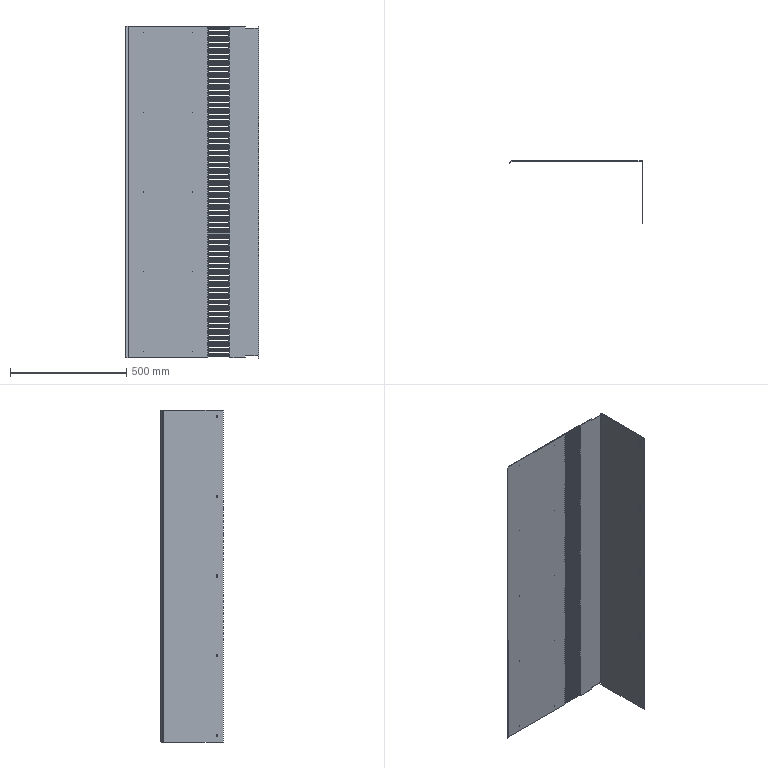Part | SolidWorks | features BaseBody 1 | 1 solid | 625 faces | box 575.794 x 268 x 1427 mm | volume 3365860 mm3 | cylinder 317 | plane 308 | commonest cylinder face diameters 6 x276 2.5 x20 5.5 x15 0.4 x2 6.4 x2 20 x2